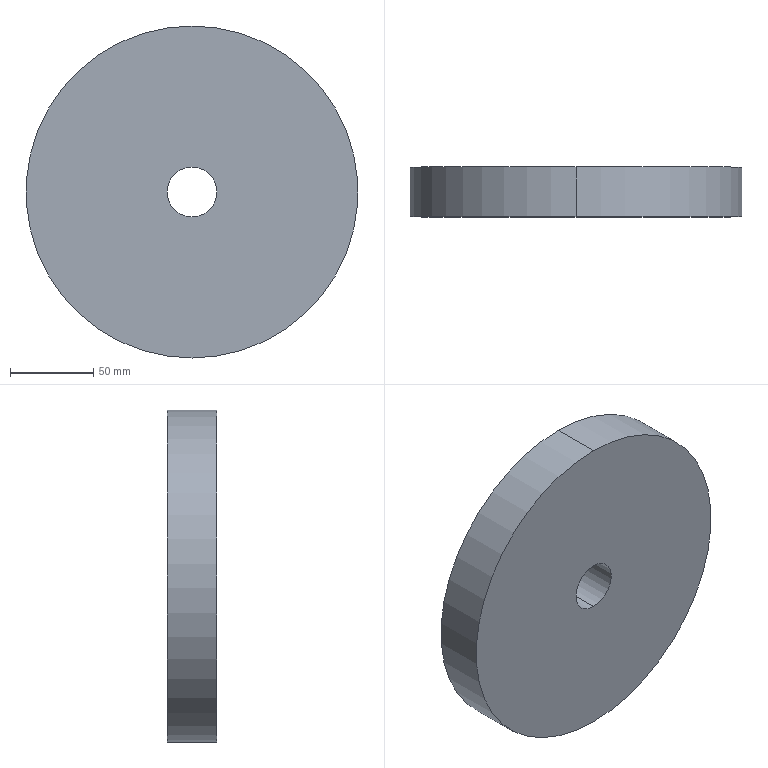Part | SolidWorks | features Revolution 1 | 1 solid | 6 faces | box 200 x 30 x 200 mm | volume 921272 mm3 | cylinder 4 | plane 2 | commonest cylinder face diameters 30 x2 200 x2
STEP:
#1=CARTESIAN_POINT('',(0.,0.,-15.));
#2=VERTEX_POINT('',#1);
#3=CARTESIAN_POINT('',(0.,0.,15.));
#4=VERTEX_POINT('',#3);
#5=CARTESIAN_POINT('',(0.,0.,0.));
#6=DIRECTION('',(0.,1.,0.));
#7=DIRECTION('',(0.,0.,1.));
#8=AXIS2_PLACEMENT_3D('',#5,#6,#7);
#9=CIRCLE('',#8,15.);
#10=EDGE_CURVE('',#2,#4,#9,.T.);
#11=ORIENTED_EDGE('',*,*,#10,.F.);
#12=CARTESIAN_POINT('',(0.,30.,-15.));
#13=VERTEX_POINT('',#12);
#14=CARTESIAN_POINT('',(0.,36.72,-15.));
#15=DIRECTION('',(0.,1.,0.));
#16=VECTOR('',#15,1000.);
#17=LINE('',#14,#16);
#18=EDGE_CURVE('',#2,#13,#17,.T.);
#19=ORIENTED_EDGE('',*,*,#18,.T.);
#20=CARTESIAN_POINT('',(0.,30.,15.));
#21=VERTEX_POINT('',#20);
#22=CARTESIAN_POINT('',(0.,30.,0.));
#23=DIRECTION('',(0.,1.,0.));
#24=DIRECTION('',(0.,0.,1.));
#25=AXIS2_PLACEMENT_3D('',#22,#23,#24);
#26=CIRCLE('',#25,15.);
#27=EDGE_CURVE('',#13,#21,#26,.T.);
#28=ORIENTED_EDGE('',*,*,#27,.T.);
#29=CARTESIAN_POINT('',(0.,36.72,15.));
#30=DIRECTION('',(0.,1.,0.));
#31=VECTOR('',#30,1000.);
#32=LINE('',#29,#31);
#33=EDGE_CURVE('',#4,#21,#32,.T.);
#34=ORIENTED_EDGE('',*,*,#33,.F.);
#35=EDGE_LOOP('',(#11,#19,#28,#34));
#36=FACE_OUTER_BOUND('',#35,.T.);
#37=CARTESIAN_POINT('',(0.,36.72,0.));
#38=DIRECTION('',(0.,1.,0.));
#39=DIRECTION('',(0.,0.,1.));
#40=AXIS2_PLACEMENT_3D('',#37,#38,#39);
#41=CYLINDRICAL_SURFACE('',#40,15.);
#42=ADVANCED_FACE('',(#36),#41,.F.);
#43=CARTESIAN_POINT('',(0.,0.,100.));
#44=VERTEX_POINT('',#43);
#45=CARTESIAN_POINT('',(0.,0.,-100.));
#46=VERTEX_POINT('',#45);
#47=CARTESIAN_POINT('',(0.,0.,0.));
#48=DIRECTION('',(0.,1.,0.));
#49=DIRECTION('',(0.,0.,1.));
#50=AXIS2_PLACEMENT_3D('',#47,#48,#49);
#51=CIRCLE('',#50,100.);
#52=EDGE_CURVE('',#44,#46,#51,.T.);
#53=ORIENTED_EDGE('',*,*,#52,.T.);
#54=CARTESIAN_POINT('',(0.,30.,-100.));
#55=VERTEX_POINT('',#54);
#56=CARTESIAN_POINT('',(0.,36.72,-100.));
#57=DIRECTION('',(0.,1.,0.));
#58=VECTOR('',#57,1000.);
#59=LINE('',#56,#58);
#60=EDGE_CURVE('',#46,#55,#59,.T.);
#61=ORIENTED_EDGE('',*,*,#60,.T.);
#62=CARTESIAN_POINT('',(0.,30.,100.));
#63=VERTEX_POINT('',#62);
#64=CARTESIAN_POINT('',(0.,30.,0.));
#65=DIRECTION('',(0.,1.,0.));
#66=DIRECTION('',(0.,0.,1.));
#67=AXIS2_PLACEMENT_3D('',#64,#65,#66);
#68=CIRCLE('',#67,100.);
#69=EDGE_CURVE('',#63,#55,#68,.T.);
#70=ORIENTED_EDGE('',*,*,#69,.F.);
#71=CARTESIAN_POINT('',(0.,36.72,100.));
#72=DIRECTION('',(0.,1.,0.));
#73=VECTOR('',#72,1000.);
#74=LINE('',#71,#73);
#75=EDGE_CURVE('',#44,#63,#74,.T.);
#76=ORIENTED_EDGE('',*,*,#75,.F.);
#77=EDGE_LOOP('',(#53,#61,#70,#76));
#78=FACE_OUTER_BOUND('',#77,.T.);
#79=CARTESIAN_POINT('',(0.,36.72,0.));
#80=DIRECTION('',(0.,1.,0.));
#81=DIRECTION('',(0.,0.,1.));
#82=AXIS2_PLACEMENT_3D('',#79,#80,#81);
#83=CYLINDRICAL_SURFACE('',#82,100.);
#84=ADVANCED_FACE('',(#78),#83,.T.);
#85=ORIENTED_EDGE('',*,*,#60,.F.);
#86=CARTESIAN_POINT('',(0.,0.,0.));
#87=DIRECTION('',(0.,1.,0.));
#88=DIRECTION('',(0.,0.,1.));
#89=AXIS2_PLACEMENT_3D('',#86,#87,#88);
#90=CIRCLE('',#89,100.);
#91=EDGE_CURVE('',#46,#44,#90,.T.);
#92=ORIENTED_EDGE('',*,*,#91,.T.);
#93=ORIENTED_EDGE('',*,*,#75,.T.);
#94=CARTESIAN_POINT('',(0.,30.,0.));
#95=DIRECTION('',(0.,1.,0.));
#96=DIRECTION('',(0.,0.,1.));
#97=AXIS2_PLACEMENT_3D('',#94,#95,#96);
#98=CIRCLE('',#97,100.);
#99=EDGE_CURVE('',#55,#63,#98,.T.);
#100=ORIENTED_EDGE('',*,*,#99,.F.);
#101=EDGE_LOOP('',(#85,#92,#93,#100));
#102=FACE_OUTER_BOUND('',#101,.T.);
#103=CARTESIAN_POINT('',(0.,36.72,0.));
#104=DIRECTION('',(0.,1.,0.));
#105=DIRECTION('',(0.,0.,1.));
#106=AXIS2_PLACEMENT_3D('',#103,#104,#105);
#107=CYLINDRICAL_SURFACE('',#106,100.);
#108=ADVANCED_FACE('',(#102),#107,.T.);
#109=CARTESIAN_POINT('',(0.,30.,0.));
#110=DIRECTION('',(0.,1.,0.));
#111=DIRECTION('',(0.,0.,1.));
#112=AXIS2_PLACEMENT_3D('',#109,#110,#111);
#113=CIRCLE('',#112,15.);
#114=EDGE_CURVE('',#21,#13,#113,.T.);
#115=ORIENTED_EDGE('',*,*,#114,.F.);
#116=ORIENTED_EDGE('',*,*,#27,.F.);
#117=EDGE_LOOP('',(#115,#116));
#118=FACE_BOUND('',#117,.T.);
#119=ORIENTED_EDGE('',*,*,#69,.T.);
#120=ORIENTED_EDGE('',*,*,#99,.T.);
#121=EDGE_LOOP('',(#119,#120));
#122=FACE_OUTER_BOUND('',#121,.T.);
#123=CARTESIAN_POINT('',(0.,30.,-100.));
#124=DIRECTION('',(0.,-1.,0.));
#125=DIRECTION('',(0.,0.,-1.));
#126=AXIS2_PLACEMENT_3D('',#123,#124,#125);
#127=PLANE('',#126);
#128=ADVANCED_FACE('',(#118,#122),#127,.F.);
#129=ORIENTED_EDGE('',*,*,#18,.F.);
#130=CARTESIAN_POINT('',(0.,0.,0.));
#131=DIRECTION('',(0.,1.,0.));
#132=DIRECTION('',(0.,0.,1.));
#133=AXIS2_PLACEMENT_3D('',#130,#131,#132);
#134=CIRCLE('',#133,15.);
#135=EDGE_CURVE('',#4,#2,#134,.T.);
#136=ORIENTED_EDGE('',*,*,#135,.F.);
#137=ORIENTED_EDGE('',*,*,#33,.T.);
#138=ORIENTED_EDGE('',*,*,#114,.T.);
#139=EDGE_LOOP('',(#129,#136,#137,#138));
#140=FACE_OUTER_BOUND('',#139,.T.);
#141=CARTESIAN_POINT('',(0.,36.72,0.));
#142=DIRECTION('',(0.,1.,0.));
#143=DIRECTION('',(0.,0.,1.));
#144=AXIS2_PLACEMENT_3D('',#141,#142,#143);
#145=CYLINDRICAL_SURFACE('',#144,15.);
#146=ADVANCED_FACE('',(#140),#145,.F.);
#147=ORIENTED_EDGE('',*,*,#52,.F.);
#148=ORIENTED_EDGE('',*,*,#91,.F.);
#149=EDGE_LOOP('',(#147,#148));
#150=FACE_OUTER_BOUND('',#149,.T.);
#151=ORIENTED_EDGE('',*,*,#135,.T.);
#152=ORIENTED_EDGE('',*,*,#10,.T.);
#153=EDGE_LOOP('',(#151,#152));
#154=FACE_BOUND('',#153,.T.);
#155=CARTESIAN_POINT('',(0.,0.,-15.));
#156=DIRECTION('',(0.,1.,0.));
#157=DIRECTION('',(0.,0.,1.));
#158=AXIS2_PLACEMENT_3D('',#155,#156,#157);
#159=PLANE('',#158);
#160=ADVANCED_FACE('',(#150,#154),#159,.F.);
#161=CLOSED_SHELL('',(#42,#84,#108,#128,#146,#160));
#162=MANIFOLD_SOLID_BREP('',#161);
#163=CARTESIAN_POINT('',(0.,0.,0.));
#164=DIRECTION('',(0.,0.,1.));
#165=DIRECTION('',(1.,0.,0.));
#166=AXIS2_PLACEMENT_3D('',#163,#164,#165);
#167=(LENGTH_UNIT()NAMED_UNIT(*)SI_UNIT(.MILLI.,.METRE.));
#168=UNCERTAINTY_MEASURE_WITH_UNIT(LENGTH_MEASURE(0.00001),#167,'','');
#169=(NAMED_UNIT(*)PLANE_ANGLE_UNIT()SI_UNIT($,.RADIAN.));
#170=(NAMED_UNIT(*)SI_UNIT($,.STERADIAN.)SOLID_ANGLE_UNIT());
#171=(GEOMETRIC_REPRESENTATION_CONTEXT(3)GLOBAL_UNCERTAINTY_ASSIGNED_CONTEXT((#168))GLOBAL_UNIT_ASSIGNED_CONTEXT((#167,#169,#170))REPRESENTATION_CONTEXT('',''));
#172=ADVANCED_BREP_SHAPE_REPRESENTATION('',(#162,#166),#171);